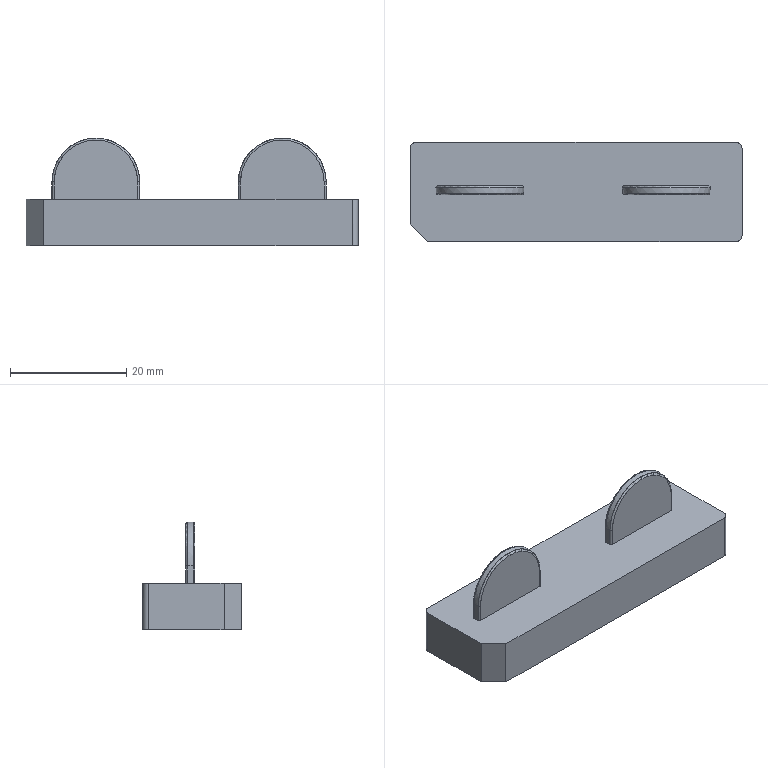NC program | PowerMill | posted by the shop | part box 57 x 17 x 18.538 mm
Lines 9851 to 10660 of 218548:
( TOOL ID   D10_1_1_1 )
( TOOL DIA. 10. TIP RAD 0 LENGTH 73.68 )
( Z = -10.74 )
T3 M6
T22
G91 G28 Z0
G0 G90 G54
M08
S8500 M3
X0 Y0 M8
G43 Z9.797 H3
X39.254 Y1.269
Z-9.54
G1 Z-10.74 F360
X33.979 F600
X28.409 Y1.009
X28.416 Y.787
X28.415 Y.564
X28.389 Y.109
X28.346 Y-.554
X28.323 Y-.82
X28.275 Y-1.145
X28.222 Y-1.421
X28.155 Y-1.694
X28.073 Y-1.963
X27.978 Y-2.227
X27.863 Y-2.506
X27.763 Y-2.719
X27.653 Y-2.928
X27.535 Y-3.132
G2 X27.231 Y-3.584 I-6.175 J3.828
G1 X27.083 Y-3.775
X26.926 Y-3.959
G2 X26.172 Y-4.667 I-4.573 J4.113
G1 X25.978 Y-4.812
X25.779 Y-4.948
G2 X25.309 Y-5.224 I-3.876 J6.075
G1 X25.098 Y-5.329
X24.882 Y-5.425
G2 X24.378 Y-5.609 I-2.324 J5.603
G1 X24.108 Y-5.688
X23.835 Y-5.752
X23.51 Y-5.809
X23.218 Y-5.844
X22.946 Y-5.865
X22.673 Y-5.872
X8.327
G2 X7.559 Y-5.817 I.024 J5.762
G1 X7.442 Y-5.802
X7.165 Y-5.752
X6.892 Y-5.688
X6.56 Y-5.589
X6.337 Y-5.512
G2 X5.318 Y-5.007 I1.952 J5.227
G1 X5.221 Y-4.948
X5.021 Y-4.812
X4.828 Y-4.667
X4.602 Y-4.48
X1.17 Y-7.858
X1.513 Y-8.206
G2 X1.11 Y-9.175 I-.404 J-.401
G1 X-2.095
G2 X-2.5 Y-8.168 I0 J.585
G1 X-2.07 Y-7.756
X-1.119 Y-6.8
G2 X.224 Y-6.847 I.65 J-.644
G1 X.599 Y-7.277
X1.17 Y-7.858
X4.602 Y-4.48
G2 X4.074 Y-3.959 I4.017 J4.605
G1 X3.917 Y-3.775
X3.769 Y-3.584
G2 X3.465 Y-3.132 I5.832 J4.255
X3.137 Y-2.506 I4.818 J2.922
G1 X3.022 Y-2.227
X2.927 Y-1.963
X2.845 Y-1.694
X2.778 Y-1.421
X2.725 Y-1.145
X2.677 Y-.82
X2.654 Y-.554
X2.594 Y.367
G2 X2.59 Y.986 I5.54 J.349
G1 X2.608 Y1.275
G2 X2.677 Y1.766 I6.024 J-.584
G1 X2.728 Y2.009
X2.809 Y2.319
X2.886 Y2.567
X2.975 Y2.81
X3.075 Y3.049
X3.186 Y3.283
X3.345 Y3.576
X3.481 Y3.801
X3.627 Y4.02
X3.784 Y4.231
X3.951 Y4.434
X4.179 Y4.682
X4.362 Y4.865
X4.554 Y5.039
X4.754 Y5.204
X4.961 Y5.359
G2 X5.449 Y5.671 I4.166 J-5.968
X5.89 Y5.899 I2.99 J-5.253
X6.415 Y6.108 I2.498 J-5.517
G1 X6.662 Y6.188
X6.913 Y6.256
X7.166 Y6.312
X7.422 Y6.356
X7.68 Y6.387
X7.939 Y6.406
X8.199 Y6.412
X22.801
X23.061 Y6.406
G2 X23.834 Y6.312 I-.305 J-5.745
G1 X24.087 Y6.256
G2 X25.11 Y5.899 I-1.492 J-5.915
G1 X25.333 Y5.79
X25.551 Y5.671
X25.763 Y5.543
G2 X26.246 Y5.204 I-3.362 J-5.315
X26.638 Y4.865 I-3.821 J-4.813
G1 X26.872 Y4.628
X27.049 Y4.434
X27.216 Y4.231
X27.373 Y4.02
X27.518 Y3.803
G2 X27.814 Y3.283 I-6.147 J-3.845
X28.025 Y2.81 I-5.662 J-2.816
G1 X28.114 Y2.567
X28.21 Y2.25
X28.272 Y2.009
G2 X28.392 Y1.275 I-5.629 J-1.29
G1 X28.409 Y1.009
X33.979 Y1.269
G0 Z2.826
G1 X-39.255 Y.233 F10000
G0 Z-9.54
G1 Z-10.74 F360
X-33.98 F600
X-29.41 Y.45
G2 X-29.409 Y1.027 I5.682 J.27
G1 X-29.392 Y1.275
X-29.363 Y1.521
G2 X-29.272 Y2.009 I5.984 J-.86
G1 X-29.191 Y2.319
X-29.114 Y2.567
X-29.025 Y2.81
X-28.925 Y3.049
X-28.814 Y3.283
X-28.655 Y3.576
X-28.519 Y3.801
X-28.373 Y4.02
X-28.216 Y4.231
X-28.049 Y4.434
G2 X-27.638 Y4.865 I5.486 J-4.813
G1 X-27.446 Y5.039
X-27.246 Y5.204
X-27.039 Y5.359
X-26.824 Y5.504
G2 X-26.333 Y5.79 I3.322 J-5.127
X-24.834 Y6.312 I2.654 J-5.213
X-24.061 Y6.406 I1.07 J-5.592
G1 X-23.801 Y6.412
X-9.199
G2 X-8.68 Y6.387 I-.048 J-6.371
G1 X-8.422 Y6.356
G2 X-7.662 Y6.188 I-.842 J-5.62
X-7.118 Y5.997 I-2.097 J-6.856
G1 X-6.89 Y5.899
X-6.667 Y5.79
G2 X-6.176 Y5.504 I-2.95 J-5.616
G1 X-5.961 Y5.359
X-5.754 Y5.204
X-5.554 Y5.039
X-5.458 Y4.953
X-1.829 Y8.148
G2 X-1.367 Y9.175 I.463 J.41
G1 X.366
G2 X.812 Y8.13 I0 J-.618
G1 X.177 Y7.467
G2 X-1.259 Y7.5 I-.703 J.674
G1 X-1.829 Y8.148
X-5.458 Y4.953
X-5.362 Y4.865
G2 X-4.951 Y4.434 I-5.049 J-5.22
G1 X-4.784 Y4.231
X-4.627 Y4.02
G2 X-4.271 Y3.441 I-4.856 J-3.389
G1 X-4.186 Y3.283
X-4.075 Y3.049
X-3.975 Y2.81
X-3.886 Y2.567
X-3.809 Y2.319
G2 X-3.637 Y1.521 I-5.523 J-1.612
G1 X-3.608 Y1.275
X-3.592 Y1.035
G2 X-3.594 Y.367 I-5.602 J-.317
G1 X-3.654 Y-.554
X-3.677 Y-.82
X-3.725 Y-1.145
X-3.778 Y-1.421
X-3.845 Y-1.694
X-3.927 Y-1.963
X-4.02 Y-2.221
G2 X-4.237 Y-2.719 I-5.658 J2.167
G1 X-4.346 Y-2.928
X-4.459 Y-3.122
X-4.63 Y-3.387
X-4.769 Y-3.584
X-4.917 Y-3.775
X-5.074 Y-3.959
G2 X-6.021 Y-4.812 I-4.429 J3.968
G1 X-6.221 Y-4.948
G2 X-6.902 Y-5.329 I-3.504 J5.465
G1 X-7.118 Y-5.425
X-7.337 Y-5.512
X-7.622 Y-5.609
G2 X-8.165 Y-5.752 I-1.897 J6.086
G1 X-8.442 Y-5.802
X-8.721 Y-5.838
G2 X-9.327 Y-5.872 I-.656 J6.298
G1 X-23.673
X-23.946 Y-5.865
X-24.218 Y-5.844
G2 X-25.108 Y-5.688 I.55 J5.726
X-25.663 Y-5.512 I1.897 J6.956
G1 X-25.888 Y-5.422
X-26.108 Y-5.324
X-26.308 Y-5.224
X-26.398 Y-5.174
G2 X-26.979 Y-4.812 I2.799 J5.141
G1 X-27.172 Y-4.667
X-27.359 Y-4.514
X-27.539 Y-4.353
G2 X-28.083 Y-3.775 I3.917 J4.231
G1 X-28.231 Y-3.584
G2 X-28.535 Y-3.132 I5.868 J4.279
G1 X-28.654 Y-2.928
X-28.763 Y-2.719
X-28.863 Y-2.506
X-28.978 Y-2.227
X-29.073 Y-1.963
X-29.155 Y-1.694
X-29.222 Y-1.421
X-29.285 Y-1.084
X-29.323 Y-.82
X-29.346 Y-.554
X-29.41 Y.45
X-33.98 Y.233
G0 Z9.797
Z10.797
X0 Y0
X-5.4 Y-4.523
Z-9.51
G1 Z-10.71 F360
G3 X-6.533 Y-4.707 I-.344 J-1.46 F600
G2 X-9.402 Y-5.502 I-2.798 J4.525
G1 X-23.642
G2 X-28.976 Y-.553 I-.028 J5.318
X-29.044 Y.546 I41.966 J3.176
X-24.379 Y6.009 I5.309 J.189
X-23.824 Y6.042 I.578 J-4.981
G1 X-16.521
X-9.218
G2 X-7.178 Y5.622 I0 J-5.156
X-3.956 Y.544 I-2.091 J-4.889
X-4.025 Y-.555 I-42.962 J2.14
X-6.533 Y-4.707 I-5.307 J.373
G3 X-7.204 Y-5.639 I.789 J-1.276
G1 X-5.482 Y-4.491
G3 X-6.617 Y-4.664 I-.358 J-1.457
G2 X-9.402 Y-5.422 I-2.715 J4.482
G1 X-23.641
G2 X-28.896 Y-.548 I-.029 J5.238
X-28.964 Y.548 I42.743 J3.226
X-24.371 Y5.929 I5.229 J.188
X-23.824 Y5.962 I.57 J-4.897
G1 X-16.521
X-9.219
G2 X-7.211 Y5.549 I.002 J-5.075
X-4.036 Y.548 I-2.059 J-4.816
X-4.104 Y-.548 I-42.812 J2.131
X-6.617 Y-4.664 I-5.228 J.366
G3 X-7.297 Y-5.59 I.777 J-1.283
G0 Z3.872
G1 X26.6 Y-4.523 F10000
G0 Z-9.51
G1 Z-10.71 F360
G3 X25.467 Y-4.707 I-.344 J-1.46 F600
G2 X22.728 Y-5.502 I-2.797 J4.524
G1 X8.305
G2 X3.024 Y-.553 I.025 J5.318
X2.956 Y.546 I41.991 J3.178
X3.068 Y1.839 I5.392 J.181
G1 X3.069 Y1.844
G2 X7.382 Y5.975 I5.198 J-1.11
X8.124 Y6.041 I.817 J-4.944
G1 X22.729 Y6.042
G2 X24.954 Y5.563 I.049 J-5.184
X28.044 Y.544 I-2.226 J-4.832
X27.975 Y-.555 I-43.025 J2.144
X25.467 Y-4.707 I-5.306 J.372
G3 X24.796 Y-5.638 I.789 J-1.276
G1 X26.515 Y-4.494
G3 X25.38 Y-4.667 I-.359 J-1.456
G2 X22.728 Y-5.422 I-2.71 J4.484
G1 X8.306
G2 X3.104 Y-.548 I.023 J5.238
X3.036 Y.548 I42.755 J3.227
X3.147 Y1.826 I5.313 J.18
X7.394 Y5.896 I5.12 J-1.092
X8.124 Y5.961 I.805 J-4.864
G1 X22.728 Y5.962
G2 X24.919 Y5.491 I.049 J-5.104
X27.964 Y.548 I-2.191 J-4.76
X27.896 Y-.548 I-42.846 J2.133
X25.38 Y-4.667 I-5.226 J.365
G3 X24.699 Y-5.591 I.776 J-1.284
G0 Z10.797
X0 Y0
Z9.797
X32.165 Y-17.547
Z-17.44
G1 Z-18.64 F360
G3 X30.054 Y-13.015 I-1.056 J2.266 F600
G1 X29.91 Y-13.082
X29.907 Y-13.083
X29.905 Y-13.084
X29.589 Y-13.21
X29.587 Y-13.211
X29.585
X29.269 Y-13.317
X29.267
X29.266 Y-13.318
X29.139 Y-13.355
X29.138
X29.137 Y-13.356
X28.948 Y-13.405
X28.946 Y-13.406
X28.944
X28.628 Y-13.474
X28.626 Y-13.475
X28.624
X28.308 Y-13.526
X28.306
X28.303 Y-13.527
X27.987 Y-13.56
X27.985
X27.983
X27.667 Y-13.577
X27.665
X27.663
X27.347 Y-13.58
X-25.45
X-25.451
X-25.452
X-25.768 Y-13.573
X-25.77
X-25.773
X-26.089 Y-13.546
X-26.091 Y-13.545
X-26.094
X-26.41 Y-13.498
X-26.413 Y-13.497
X-26.415
X-26.731 Y-13.429
X-26.734 Y-13.428
X-26.736 Y-13.427
X-26.994 Y-13.355
X-26.997 Y-13.354
X-27.
X-27.373 Y-13.222
X-27.376 Y-13.221
X-27.379 Y-13.22
X-27.695 Y-13.081
X-27.696
X-27.698 Y-13.08
X-27.792 Y-13.034
X-27.793 Y-13.033
X-27.794 Y-13.032
X-28.017 Y-12.913
X-28.019 Y-12.911
X-28.021 Y-12.91
X-28.337 Y-12.714
X-28.34 Y-12.712
X-28.342 Y-12.71
X-28.658 Y-12.479
X-28.66 Y-12.477
X-28.662 Y-12.476
X-28.765 Y-12.392
X-28.766 Y-12.391
X-28.768 Y-12.389
X-28.98 Y-12.2
X-28.982 Y-12.199
X-28.983 Y-12.198
X-29.113 Y-12.071
X-29.114 Y-12.07
X-32.145 Y-9.038
X-32.146 Y-9.037
X-32.147 Y-9.036
X-32.268 Y-8.907
X-32.27 Y-8.905
X-32.271 Y-8.904
X-32.466 Y-8.675
X-32.467 Y-8.673
X-32.468 Y-8.672
X-32.536 Y-8.585
X-32.537 Y-8.584
X-32.538 Y-8.582
X-32.761 Y-8.266
X-32.763 Y-8.263
X-32.764 Y-8.261
X-32.953 Y-7.945
X-32.954 Y-7.942
X-32.956 Y-7.94
X-33.109 Y-7.637
X-33.11 Y-7.634
X-33.111 Y-7.632
X-33.249 Y-7.302
X-33.251 Y-7.3
Y-7.297
X-33.359 Y-6.981
X-33.36 Y-6.979
X-33.361 Y-6.976
X-33.43 Y-6.723
X-33.431 Y-6.721
X-33.432 Y-6.718
X-33.51 Y-6.339
X-33.511 Y-6.336
Y-6.334
X-33.554 Y-6.017
Y-6.015
Y-6.012
X-33.576 Y-5.696
Y-5.694
Y-5.692
X-33.58 Y-5.375
Y-5.374
X-33.579 Y7.588
Y7.589
Y7.591
X-33.566 Y7.907
Y7.909
Y7.911
X-33.536 Y8.227
Y8.229
Y8.231
X-33.489 Y8.548
Y8.55
X-33.488 Y8.552
X-33.432 Y8.834
X-33.431 Y8.836
Y8.838
X-33.341 Y9.188
X-33.34 Y9.19
Y9.193
X-33.238 Y9.509
Y9.511
X-33.237 Y9.513
X-33.116 Y9.829
X-33.115 Y9.831
X-33.114 Y9.833
X-32.972 Y10.149
X-32.971 Y10.152
X-32.97 Y10.154
X-32.805 Y10.47
X-32.804 Y10.472
X-32.803 Y10.474
X-32.613 Y10.79
X-32.612 Y10.792
X-32.61 Y10.794
X-32.471 Y11.
Y11.001
X-32.47 Y11.003
X-32.391 Y11.112
X-32.39 Y11.113
X-32.389 Y11.115
X-32.152 Y11.415
X-32.15 Y11.417
X-32.148 Y11.419
X-31.847 Y11.751
X-31.844 Y11.753
X-31.842 Y11.755
X-31.511 Y12.069
X-31.509 Y12.071
X-31.507 Y12.072
X-31.191 Y12.331
X-31.19 Y12.332
X-31.188 Y12.333
X-31.108 Y12.394
X-31.107 Y12.395
X-31.106
X-30.87 Y12.56
X-30.868 Y12.561
X-30.867 Y12.562
X-30.55 Y12.759
X-30.548 Y12.761
X-30.546 Y12.762
X-30.23 Y12.933
X-30.228 Y12.934
X-30.226 Y12.935
X-29.91 Y13.082
X-29.907 Y13.083
X-29.905 Y13.084
X-29.589 Y13.21
X-29.587 Y13.211
X-29.585
X-29.269 Y13.317
X-29.267 Y13.318
X-29.265
X-28.948 Y13.405
X-28.946
X-28.944 Y13.406
X-28.628 Y13.474
X-28.626 Y13.475
X-28.624
X-28.308 Y13.526
X-28.306
X-28.303 Y13.527
X-27.987 Y13.56
X-27.985
X-27.983
X-27.667 Y13.577
X-27.665
X-27.663
X-27.347 Y13.58
X0
X27.347
X27.663 Y13.577
X27.665
X27.667
X27.983 Y13.561
X27.985
X27.987 Y13.56
X28.304 Y13.527
X28.306 Y13.526
X28.308
X28.624 Y13.475
X28.626
X28.628 Y13.474
X28.944 Y13.406
X28.946 Y13.405
X28.948
X29.265 Y13.318
X29.267
X29.269 Y13.317
X29.585 Y13.211
X29.587 Y13.21
X29.589 Y13.209
X29.905 Y13.084
X29.907 Y13.083
X29.91 Y13.082
X30.226 Y12.934
X30.228 Y12.933
X30.23 Y12.932
X30.546 Y12.762
X30.548 Y12.761
X30.55 Y12.759
X30.866 Y12.563
X30.869 Y12.562
X30.871 Y12.56
X31.187 Y12.335
X31.189 Y12.333
X31.191 Y12.331
X31.504 Y12.075
X31.506 Y12.074
X31.508 Y12.072
X31.828 Y11.771
X31.83 Y11.768
X31.832 Y11.766
X32.134 Y11.435
X32.136 Y11.433
X32.138 Y11.431
X32.389 Y11.115
X32.39 Y11.113
X32.391 Y11.112
X32.47 Y11.002
X32.471 Y11.001
Y11.
X32.61 Y10.794
X32.611 Y10.792
X32.612 Y10.79
X32.79 Y10.498
X32.791 Y10.496
X32.792 Y10.494
X32.97 Y10.154
X32.971 Y10.152
X32.972 Y10.15
X33.11 Y9.844
X33.111 Y9.841
X33.112 Y9.839
X33.237 Y9.513
X33.238 Y9.511
Y9.509
X33.34 Y9.193
Y9.19
X33.341 Y9.188
X33.423 Y8.872
X33.424 Y8.87
Y8.868
X33.488 Y8.552
Y8.55
Y8.548
X33.536 Y8.232
Y8.229
Y8.227
X33.565 Y7.911
Y7.909
X33.566 Y7.907
X33.579 Y7.591
Y7.589
Y7.587
Y-7.587
Y-7.589
Y-7.591
X33.566 Y-7.907
Y-7.909
Y-7.911
X33.536 Y-8.227
Y-8.229
Y-8.231
X33.489 Y-8.548
Y-8.55
X33.488 Y-8.552
X33.432 Y-8.834
X33.431 Y-8.836
Y-8.838
X33.341 Y-9.188
X33.34 Y-9.19
Y-9.193
X33.238 Y-9.509
Y-9.511
X33.237 Y-9.513
X33.116 Y-9.829
X33.115 Y-9.831
X33.114 Y-9.833
X32.972 Y-10.149
X32.971 Y-10.152
X32.97 Y-10.154
X32.805 Y-10.47
X32.804 Y-10.472
X32.803 Y-10.474
X32.613 Y-10.79
X32.612 Y-10.792
X32.61 Y-10.794
X32.471 Y-11.
Y-11.001
X32.47 Y-11.003
X32.391 Y-11.112
X32.39 Y-11.113
X32.389 Y-11.115
X32.152 Y-11.415
X32.15 Y-11.417
X32.148 Y-11.419
X31.847 Y-11.751
X31.844 Y-11.753
X31.842 Y-11.755
X31.511 Y-12.069
X31.509 Y-12.071
X31.507 Y-12.072
X31.191 Y-12.331
X31.19 Y-12.332
X31.188 Y-12.333
X31.108 Y-12.394
X31.107 Y-12.395
X31.106
X30.87 Y-12.56
X30.868 Y-12.561
X30.867 Y-12.562
X30.55 Y-12.759
X30.548 Y-12.761
X30.546 Y-12.762
X30.23 Y-12.933
X30.228 Y-12.934
X30.226 Y-12.935
X30.054 Y-13.015
G3 X32.165 Y-17.547 I1.056 J-2.266
G1 X32.119 Y-17.48
G3 X30.008 Y-12.948 I-1.056 J2.266
G1 X29.876 Y-13.01
X29.56 Y-13.135
X29.243 Y-13.241
X29.116 Y-13.278
X28.927 Y-13.328
X28.611 Y-13.396
X28.295 Y-13.447
X27.979 Y-13.481
X27.663 Y-13.497
X27.347 Y-13.5
X-25.45
X-25.766 Y-13.493
X-26.082 Y-13.466
X-26.398 Y-13.419
X-26.714 Y-13.35
X-26.973 Y-13.278
X-27.347 Y-13.147
X-27.663 Y-13.008
X-27.756 Y-12.962
X-27.979 Y-12.842
X-28.295 Y-12.646
X-28.611 Y-12.414
X-28.715 Y-12.33
X-28.927 Y-12.141
X-29.058 Y-12.014
X-32.089 Y-8.981
X-32.21 Y-8.852
X-32.405 Y-8.623
X-32.473 Y-8.536
X-32.696 Y-8.22
X-32.884 Y-7.904
X-33.037 Y-7.601
X-33.176 Y-7.271
X-33.284 Y-6.955
X-33.353 Y-6.702
X-33.432 Y-6.323
X-33.474 Y-6.007
X-33.496 Y-5.691
X-33.5 Y-5.374
Y7.271
X-33.499 Y7.587
X-33.486 Y7.904
X-33.457 Y8.22
X-33.41 Y8.536
X-33.353 Y8.818
X-33.263 Y9.168
X-33.162 Y9.484
X-33.041 Y9.801
X-32.899 Y10.117
X-32.734 Y10.433
X-32.544 Y10.749
X-32.405 Y10.956
X-32.326 Y11.065
X-32.089 Y11.366
X-31.787 Y11.697
X-31.456 Y12.011
X-31.14 Y12.269
X-31.06 Y12.33
X-30.824 Y12.494
X-30.508 Y12.692
X-30.192 Y12.862
X-29.876 Y13.01
X-29.56 Y13.135
X-29.243 Y13.241
X-28.927 Y13.328
X-28.611 Y13.396
X-28.295 Y13.447
X-27.979 Y13.481
X-27.663 Y13.497
X-27.347 Y13.5
X0
X27.347
X27.663 Y13.497
X27.979 Y13.481
X28.295 Y13.447
X28.611 Y13.396
X28.927 Y13.328
X29.243 Y13.241
X29.56 Y13.135
X29.876 Y13.01
X30.192 Y12.862
X30.508 Y12.692
X30.824 Y12.495
X31.14 Y12.269
X31.453 Y12.014
X31.773 Y11.712
X32.075 Y11.381
X32.326 Y11.065
X32.405 Y10.955
X32.544 Y10.749
X32.721 Y10.456
X32.899 Y10.117
X33.037 Y9.811
X33.162 Y9.484
X33.263 Y9.168
X33.346 Y8.852
X33.409 Y8.536
X33.457 Y8.22
X33.486 Y7.904
X33.499 Y7.587
X33.5 Y7.271
Y-7.271
X33.499 Y-7.587
X33.486 Y-7.904
X33.457 Y-8.22
X33.41 Y-8.536
X33.353 Y-8.818
X33.263 Y-9.168
X33.162 Y-9.484
X33.041 Y-9.801
X32.899 Y-10.117
X32.734 Y-10.433
X32.544 Y-10.749
X32.405 Y-10.956
X32.326 Y-11.065
X32.089 Y-11.366
X31.787 Y-11.697
X31.456 Y-12.011
X31.14 Y-12.269
X31.06 Y-12.33
X30.824 Y-12.494
X30.508 Y-12.692
X30.192 Y-12.862
X30.008 Y-12.948
G3 X32.119 Y-17.48 I1.056 J-2.266
G0 Z9.797
Z10.797
X0 Y0
M9
M5
M01